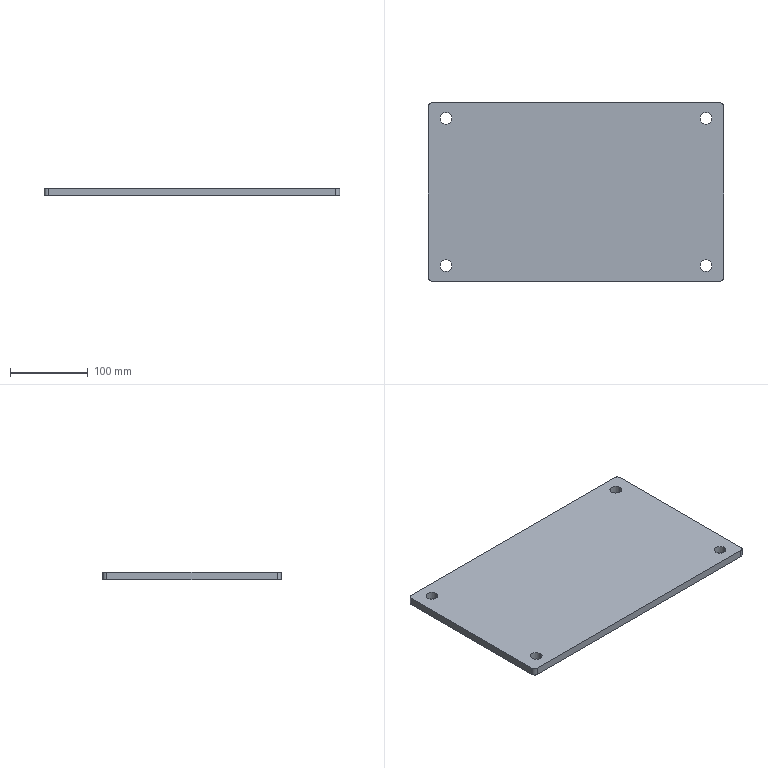Part | SolidWorks | features Chamfer 1, Extrusion 1, Fillet 1, HoleWzd 1 | 1 solid | 18 faces | box 381 x 230 x 10 mm | volume 869017 mm3 | cylinder 12 | plane 6 | commonest cylinder face diameters 15 x8 10 x4
STEP:
#1=CARTESIAN_POINT('',(-175.,95.,-5.));
#2=VERTEX_POINT('',#1);
#3=CARTESIAN_POINT('',(-160.,95.,-5.));
#4=VERTEX_POINT('',#3);
#5=CARTESIAN_POINT('',(-167.5,95.,-5.));
#6=DIRECTION('',(0.,0.,1.));
#7=DIRECTION('',(1.,0.,0.));
#8=AXIS2_PLACEMENT_3D('',#5,#6,#7);
#9=CIRCLE('',#8,7.5);
#10=EDGE_CURVE('',#2,#4,#9,.T.);
#11=ORIENTED_EDGE('',*,*,#10,.F.);
#12=CARTESIAN_POINT('',(-175.,95.,5.));
#13=VERTEX_POINT('',#12);
#14=CARTESIAN_POINT('',(-175.,95.,5.));
#15=DIRECTION('',(0.,0.,1.));
#16=VECTOR('',#15,1000.);
#17=LINE('',#14,#16);
#18=EDGE_CURVE('',#2,#13,#17,.T.);
#19=ORIENTED_EDGE('',*,*,#18,.T.);
#20=CARTESIAN_POINT('',(-160.,95.,5.));
#21=VERTEX_POINT('',#20);
#22=CARTESIAN_POINT('',(-167.5,95.,5.));
#23=DIRECTION('',(0.,0.,1.));
#24=DIRECTION('',(1.,0.,0.));
#25=AXIS2_PLACEMENT_3D('',#22,#23,#24);
#26=CIRCLE('',#25,7.5);
#27=EDGE_CURVE('',#13,#21,#26,.T.);
#28=ORIENTED_EDGE('',*,*,#27,.T.);
#29=CARTESIAN_POINT('',(-160.,95.,5.));
#30=DIRECTION('',(0.,0.,1.));
#31=VECTOR('',#30,1000.);
#32=LINE('',#29,#31);
#33=EDGE_CURVE('',#4,#21,#32,.T.);
#34=ORIENTED_EDGE('',*,*,#33,.F.);
#35=EDGE_LOOP('',(#11,#19,#28,#34));
#36=FACE_OUTER_BOUND('',#35,.T.);
#37=CARTESIAN_POINT('',(-167.5,95.,5.));
#38=DIRECTION('',(0.,0.,1.));
#39=DIRECTION('',(1.,0.,0.));
#40=AXIS2_PLACEMENT_3D('',#37,#38,#39);
#41=CYLINDRICAL_SURFACE('',#40,7.5);
#42=ADVANCED_FACE('',(#36),#41,.F.);
#43=CARTESIAN_POINT('',(160.,95.,-5.));
#44=VERTEX_POINT('',#43);
#45=CARTESIAN_POINT('',(175.,95.,-5.));
#46=VERTEX_POINT('',#45);
#47=CARTESIAN_POINT('',(167.5,95.,-5.));
#48=DIRECTION('',(0.,0.,1.));
#49=DIRECTION('',(1.,0.,0.));
#50=AXIS2_PLACEMENT_3D('',#47,#48,#49);
#51=CIRCLE('',#50,7.5);
#52=EDGE_CURVE('',#44,#46,#51,.T.);
#53=ORIENTED_EDGE('',*,*,#52,.F.);
#54=CARTESIAN_POINT('',(160.,95.,5.));
#55=VERTEX_POINT('',#54);
#56=CARTESIAN_POINT('',(160.,95.,5.));
#57=DIRECTION('',(0.,0.,1.));
#58=VECTOR('',#57,1000.);
#59=LINE('',#56,#58);
#60=EDGE_CURVE('',#44,#55,#59,.T.);
#61=ORIENTED_EDGE('',*,*,#60,.T.);
#62=CARTESIAN_POINT('',(175.,95.,5.));
#63=VERTEX_POINT('',#62);
#64=CARTESIAN_POINT('',(167.5,95.,5.));
#65=DIRECTION('',(0.,0.,1.));
#66=DIRECTION('',(1.,0.,0.));
#67=AXIS2_PLACEMENT_3D('',#64,#65,#66);
#68=CIRCLE('',#67,7.5);
#69=EDGE_CURVE('',#55,#63,#68,.T.);
#70=ORIENTED_EDGE('',*,*,#69,.T.);
#71=CARTESIAN_POINT('',(175.,95.,5.));
#72=DIRECTION('',(0.,0.,1.));
#73=VECTOR('',#72,1000.);
#74=LINE('',#71,#73);
#75=EDGE_CURVE('',#46,#63,#74,.T.);
#76=ORIENTED_EDGE('',*,*,#75,.F.);
#77=EDGE_LOOP('',(#53,#61,#70,#76));
#78=FACE_OUTER_BOUND('',#77,.T.);
#79=CARTESIAN_POINT('',(167.5,95.,5.));
#80=DIRECTION('',(0.,0.,1.));
#81=DIRECTION('',(1.,0.,0.));
#82=AXIS2_PLACEMENT_3D('',#79,#80,#81);
#83=CYLINDRICAL_SURFACE('',#82,7.5);
#84=ADVANCED_FACE('',(#78),#83,.F.);
#85=CARTESIAN_POINT('',(160.,-95.,-5.));
#86=VERTEX_POINT('',#85);
#87=CARTESIAN_POINT('',(175.,-95.,-5.));
#88=VERTEX_POINT('',#87);
#89=CARTESIAN_POINT('',(167.5,-95.,-5.));
#90=DIRECTION('',(0.,0.,1.));
#91=DIRECTION('',(1.,0.,0.));
#92=AXIS2_PLACEMENT_3D('',#89,#90,#91);
#93=CIRCLE('',#92,7.5);
#94=EDGE_CURVE('',#86,#88,#93,.T.);
#95=ORIENTED_EDGE('',*,*,#94,.F.);
#96=CARTESIAN_POINT('',(160.,-95.,5.));
#97=VERTEX_POINT('',#96);
#98=CARTESIAN_POINT('',(160.,-95.,5.));
#99=DIRECTION('',(0.,0.,1.));
#100=VECTOR('',#99,1000.);
#101=LINE('',#98,#100);
#102=EDGE_CURVE('',#86,#97,#101,.T.);
#103=ORIENTED_EDGE('',*,*,#102,.T.);
#104=CARTESIAN_POINT('',(175.,-95.,5.));
#105=VERTEX_POINT('',#104);
#106=CARTESIAN_POINT('',(167.5,-95.,5.));
#107=DIRECTION('',(0.,0.,1.));
#108=DIRECTION('',(1.,0.,0.));
#109=AXIS2_PLACEMENT_3D('',#106,#107,#108);
#110=CIRCLE('',#109,7.5);
#111=EDGE_CURVE('',#97,#105,#110,.T.);
#112=ORIENTED_EDGE('',*,*,#111,.T.);
#113=CARTESIAN_POINT('',(175.,-95.,5.));
#114=DIRECTION('',(0.,0.,1.));
#115=VECTOR('',#114,1000.);
#116=LINE('',#113,#115);
#117=EDGE_CURVE('',#88,#105,#116,.T.);
#118=ORIENTED_EDGE('',*,*,#117,.F.);
#119=EDGE_LOOP('',(#95,#103,#112,#118));
#120=FACE_OUTER_BOUND('',#119,.T.);
#121=CARTESIAN_POINT('',(167.5,-95.,5.));
#122=DIRECTION('',(0.,0.,1.));
#123=DIRECTION('',(1.,0.,0.));
#124=AXIS2_PLACEMENT_3D('',#121,#122,#123);
#125=CYLINDRICAL_SURFACE('',#124,7.5);
#126=ADVANCED_FACE('',(#120),#125,.F.);
#127=CARTESIAN_POINT('',(-175.,-95.,-5.));
#128=VERTEX_POINT('',#127);
#129=CARTESIAN_POINT('',(-160.,-95.,-5.));
#130=VERTEX_POINT('',#129);
#131=CARTESIAN_POINT('',(-167.5,-95.,-5.));
#132=DIRECTION('',(0.,0.,1.));
#133=DIRECTION('',(1.,0.,0.));
#134=AXIS2_PLACEMENT_3D('',#131,#132,#133);
#135=CIRCLE('',#134,7.5);
#136=EDGE_CURVE('',#128,#130,#135,.T.);
#137=ORIENTED_EDGE('',*,*,#136,.F.);
#138=CARTESIAN_POINT('',(-175.,-95.,5.));
#139=VERTEX_POINT('',#138);
#140=CARTESIAN_POINT('',(-175.,-95.,5.));
#141=DIRECTION('',(0.,0.,1.));
#142=VECTOR('',#141,1000.);
#143=LINE('',#140,#142);
#144=EDGE_CURVE('',#128,#139,#143,.T.);
#145=ORIENTED_EDGE('',*,*,#144,.T.);
#146=CARTESIAN_POINT('',(-160.,-95.,5.));
#147=VERTEX_POINT('',#146);
#148=CARTESIAN_POINT('',(-167.5,-95.,5.));
#149=DIRECTION('',(0.,0.,1.));
#150=DIRECTION('',(1.,0.,0.));
#151=AXIS2_PLACEMENT_3D('',#148,#149,#150);
#152=CIRCLE('',#151,7.5);
#153=EDGE_CURVE('',#139,#147,#152,.T.);
#154=ORIENTED_EDGE('',*,*,#153,.T.);
#155=CARTESIAN_POINT('',(-160.,-95.,5.));
#156=DIRECTION('',(0.,0.,1.));
#157=VECTOR('',#156,1000.);
#158=LINE('',#155,#157);
#159=EDGE_CURVE('',#130,#147,#158,.T.);
#160=ORIENTED_EDGE('',*,*,#159,.F.);
#161=EDGE_LOOP('',(#137,#145,#154,#160));
#162=FACE_OUTER_BOUND('',#161,.T.);
#163=CARTESIAN_POINT('',(-167.5,-95.,5.));
#164=DIRECTION('',(0.,0.,1.));
#165=DIRECTION('',(1.,0.,0.));
#166=AXIS2_PLACEMENT_3D('',#163,#164,#165);
#167=CYLINDRICAL_SURFACE('',#166,7.5);
#168=ADVANCED_FACE('',(#162),#167,.F.);
#169=CARTESIAN_POINT('',(-190.5,110.,-5.));
#170=VERTEX_POINT('',#169);
#171=CARTESIAN_POINT('',(-190.5,-110.,-5.));
#172=VERTEX_POINT('',#171);
#173=CARTESIAN_POINT('',(-190.5,-115.,-5.));
#174=DIRECTION('',(0.,-1.,0.));
#175=VECTOR('',#174,1000.);
#176=LINE('',#173,#175);
#177=EDGE_CURVE('',#170,#172,#176,.T.);
#178=ORIENTED_EDGE('',*,*,#177,.T.);
#179=CARTESIAN_POINT('',(-190.5,-110.,5.));
#180=VERTEX_POINT('',#179);
#181=CARTESIAN_POINT('',(-190.5,-110.,5.));
#182=DIRECTION('',(0.,0.,1.));
#183=VECTOR('',#182,1000.);
#184=LINE('',#181,#183);
#185=EDGE_CURVE('',#172,#180,#184,.T.);
#186=ORIENTED_EDGE('',*,*,#185,.T.);
#187=CARTESIAN_POINT('',(-190.5,110.,5.));
#188=VERTEX_POINT('',#187);
#189=CARTESIAN_POINT('',(-190.5,-115.,5.));
#190=DIRECTION('',(0.,-1.,0.));
#191=VECTOR('',#190,1000.);
#192=LINE('',#189,#191);
#193=EDGE_CURVE('',#188,#180,#192,.T.);
#194=ORIENTED_EDGE('',*,*,#193,.F.);
#195=CARTESIAN_POINT('',(-190.5,110.,5.));
#196=DIRECTION('',(0.,0.,-1.));
#197=VECTOR('',#196,1000.);
#198=LINE('',#195,#197);
#199=EDGE_CURVE('',#188,#170,#198,.T.);
#200=ORIENTED_EDGE('',*,*,#199,.T.);
#201=EDGE_LOOP('',(#178,#186,#194,#200));
#202=FACE_OUTER_BOUND('',#201,.T.);
#203=CARTESIAN_POINT('',(-190.5,-115.,5.));
#204=DIRECTION('',(1.,0.,0.));
#205=DIRECTION('',(0.,0.,-1.));
#206=AXIS2_PLACEMENT_3D('',#203,#204,#205);
#207=PLANE('',#206);
#208=ADVANCED_FACE('',(#202),#207,.F.);
#209=CARTESIAN_POINT('',(-185.5,-115.,-5.));
#210=VERTEX_POINT('',#209);
#211=CARTESIAN_POINT('',(185.5,-115.,-5.));
#212=VERTEX_POINT('',#211);
#213=CARTESIAN_POINT('',(190.5,-115.,-5.));
#214=DIRECTION('',(1.,0.,0.));
#215=VECTOR('',#214,1000.);
#216=LINE('',#213,#215);
#217=EDGE_CURVE('',#210,#212,#216,.T.);
#218=ORIENTED_EDGE('',*,*,#217,.T.);
#219=CARTESIAN_POINT('',(185.5,-115.,5.));
#220=VERTEX_POINT('',#219);
#221=CARTESIAN_POINT('',(185.5,-115.,5.));
#222=DIRECTION('',(0.,0.,1.));
#223=VECTOR('',#222,1000.);
#224=LINE('',#221,#223);
#225=EDGE_CURVE('',#212,#220,#224,.T.);
#226=ORIENTED_EDGE('',*,*,#225,.T.);
#227=CARTESIAN_POINT('',(-185.5,-115.,5.));
#228=VERTEX_POINT('',#227);
#229=CARTESIAN_POINT('',(190.5,-115.,5.));
#230=DIRECTION('',(1.,0.,0.));
#231=VECTOR('',#230,1000.);
#232=LINE('',#229,#231);
#233=EDGE_CURVE('',#228,#220,#232,.T.);
#234=ORIENTED_EDGE('',*,*,#233,.F.);
#235=CARTESIAN_POINT('',(-185.5,-115.,5.));
#236=DIRECTION('',(0.,0.,-1.));
#237=VECTOR('',#236,1000.);
#238=LINE('',#235,#237);
#239=EDGE_CURVE('',#228,#210,#238,.T.);
#240=ORIENTED_EDGE('',*,*,#239,.T.);
#241=EDGE_LOOP('',(#218,#226,#234,#240));
#242=FACE_OUTER_BOUND('',#241,.T.);
#243=CARTESIAN_POINT('',(190.5,-115.,5.));
#244=DIRECTION('',(0.,1.,0.));
#245=DIRECTION('',(-1.,0.,0.));
#246=AXIS2_PLACEMENT_3D('',#243,#244,#245);
#247=PLANE('',#246);
#248=ADVANCED_FACE('',(#242),#247,.F.);
#249=CARTESIAN_POINT('',(190.5,-110.,-5.));
#250=VERTEX_POINT('',#249);
#251=CARTESIAN_POINT('',(190.5,110.,-5.));
#252=VERTEX_POINT('',#251);
#253=CARTESIAN_POINT('',(190.5,-115.,-5.));
#254=DIRECTION('',(0.,1.,0.));
#255=VECTOR('',#254,1000.);
#256=LINE('',#253,#255);
#257=EDGE_CURVE('',#250,#252,#256,.T.);
#258=ORIENTED_EDGE('',*,*,#257,.T.);
#259=CARTESIAN_POINT('',(190.5,110.,5.));
#260=VERTEX_POINT('',#259);
#261=CARTESIAN_POINT('',(190.5,110.,5.));
#262=DIRECTION('',(0.,0.,1.));
#263=VECTOR('',#262,1000.);
#264=LINE('',#261,#263);
#265=EDGE_CURVE('',#252,#260,#264,.T.);
#266=ORIENTED_EDGE('',*,*,#265,.T.);
#267=CARTESIAN_POINT('',(190.5,-110.,5.));
#268=VERTEX_POINT('',#267);
#269=CARTESIAN_POINT('',(190.5,-115.,5.));
#270=DIRECTION('',(0.,1.,0.));
#271=VECTOR('',#270,1000.);
#272=LINE('',#269,#271);
#273=EDGE_CURVE('',#268,#260,#272,.T.);
#274=ORIENTED_EDGE('',*,*,#273,.F.);
#275=CARTESIAN_POINT('',(190.5,-110.,5.));
#276=DIRECTION('',(0.,0.,-1.));
#277=VECTOR('',#276,1000.);
#278=LINE('',#275,#277);
#279=EDGE_CURVE('',#268,#250,#278,.T.);
#280=ORIENTED_EDGE('',*,*,#279,.T.);
#281=EDGE_LOOP('',(#258,#266,#274,#280));
#282=FACE_OUTER_BOUND('',#281,.T.);
#283=CARTESIAN_POINT('',(190.5,-115.,5.));
#284=DIRECTION('',(-1.,0.,0.));
#285=DIRECTION('',(0.,0.,1.));
#286=AXIS2_PLACEMENT_3D('',#283,#284,#285);
#287=PLANE('',#286);
#288=ADVANCED_FACE('',(#282),#287,.F.);
#289=CARTESIAN_POINT('',(185.5,115.,5.));
#290=VERTEX_POINT('',#289);
#291=CARTESIAN_POINT('',(-185.5,115.,5.));
#292=VERTEX_POINT('',#291);
#293=CARTESIAN_POINT('',(190.5,115.,5.));
#294=DIRECTION('',(-1.,0.,0.));
#295=VECTOR('',#294,1000.);
#296=LINE('',#293,#295);
#297=EDGE_CURVE('',#290,#292,#296,.T.);
#298=ORIENTED_EDGE('',*,*,#297,.F.);
#299=CARTESIAN_POINT('',(185.5,115.,-5.));
#300=VERTEX_POINT('',#299);
#301=CARTESIAN_POINT('',(185.5,115.,5.));
#302=DIRECTION('',(0.,0.,-1.));
#303=VECTOR('',#302,1000.);
#304=LINE('',#301,#303);
#305=EDGE_CURVE('',#290,#300,#304,.T.);
#306=ORIENTED_EDGE('',*,*,#305,.T.);
#307=CARTESIAN_POINT('',(-185.5,115.,-5.));
#308=VERTEX_POINT('',#307);
#309=CARTESIAN_POINT('',(190.5,115.,-5.));
#310=DIRECTION('',(-1.,0.,0.));
#311=VECTOR('',#310,1000.);
#312=LINE('',#309,#311);
#313=EDGE_CURVE('',#300,#308,#312,.T.);
#314=ORIENTED_EDGE('',*,*,#313,.T.);
#315=CARTESIAN_POINT('',(-185.5,115.,5.));
#316=DIRECTION('',(0.,0.,1.));
#317=VECTOR('',#316,1000.);
#318=LINE('',#315,#317);
#319=EDGE_CURVE('',#308,#292,#318,.T.);
#320=ORIENTED_EDGE('',*,*,#319,.T.);
#321=EDGE_LOOP('',(#298,#306,#314,#320));
#322=FACE_OUTER_BOUND('',#321,.T.);
#323=CARTESIAN_POINT('',(190.5,115.,5.));
#324=DIRECTION('',(0.,-1.,0.));
#325=DIRECTION('',(1.,0.,0.));
#326=AXIS2_PLACEMENT_3D('',#323,#324,#325);
#327=PLANE('',#326);
#328=ADVANCED_FACE('',(#322),#327,.F.);
#329=CARTESIAN_POINT('',(-167.5,95.,5.));
#330=DIRECTION('',(0.,0.,1.));
#331=DIRECTION('',(1.,0.,0.));
#332=AXIS2_PLACEMENT_3D('',#329,#330,#331);
#333=CIRCLE('',#332,7.5);
#334=EDGE_CURVE('',#21,#13,#333,.T.);
#335=ORIENTED_EDGE('',*,*,#334,.F.);
#336=ORIENTED_EDGE('',*,*,#27,.F.);
#337=EDGE_LOOP('',(#335,#336));
#338=FACE_BOUND('',#337,.T.);
#339=CARTESIAN_POINT('',(167.5,95.,5.));
#340=DIRECTION('',(0.,0.,1.));
#341=DIRECTION('',(1.,0.,0.));
#342=AXIS2_PLACEMENT_3D('',#339,#340,#341);
#343=CIRCLE('',#342,7.5);
#344=EDGE_CURVE('',#63,#55,#343,.T.);
#345=ORIENTED_EDGE('',*,*,#344,.F.);
#346=ORIENTED_EDGE('',*,*,#69,.F.);
#347=EDGE_LOOP('',(#345,#346));
#348=FACE_BOUND('',#347,.T.);
#349=CARTESIAN_POINT('',(167.5,-95.,5.));
#350=DIRECTION('',(0.,0.,1.));
#351=DIRECTION('',(1.,0.,0.));
#352=AXIS2_PLACEMENT_3D('',#349,#350,#351);
#353=CIRCLE('',#352,7.5);
#354=EDGE_CURVE('',#105,#97,#353,.T.);
#355=ORIENTED_EDGE('',*,*,#354,.F.);
#356=ORIENTED_EDGE('',*,*,#111,.F.);
#357=EDGE_LOOP('',(#355,#356));
#358=FACE_BOUND('',#357,.T.);
#359=CARTESIAN_POINT('',(-167.5,-95.,5.));
#360=DIRECTION('',(0.,0.,1.));
#361=DIRECTION('',(1.,0.,0.));
#362=AXIS2_PLACEMENT_3D('',#359,#360,#361);
#363=CIRCLE('',#362,7.5);
#364=EDGE_CURVE('',#147,#139,#363,.T.);
#365=ORIENTED_EDGE('',*,*,#364,.F.);
#366=ORIENTED_EDGE('',*,*,#153,.F.);
#367=EDGE_LOOP('',(#365,#366));
#368=FACE_BOUND('',#367,.T.);
#369=ORIENTED_EDGE('',*,*,#273,.T.);
#370=CARTESIAN_POINT('',(185.5,110.,5.));
#371=DIRECTION('',(0.,0.,1.));
#372=DIRECTION('',(1.,0.,0.));
#373=AXIS2_PLACEMENT_3D('',#370,#371,#372);
#374=CIRCLE('',#373,5.);
#375=EDGE_CURVE('',#260,#290,#374,.T.);
#376=ORIENTED_EDGE('',*,*,#375,.T.);
#377=ORIENTED_EDGE('',*,*,#297,.T.);
#378=CARTESIAN_POINT('',(-185.5,110.,5.));
#379=DIRECTION('',(0.,0.,1.));
#380=DIRECTION('',(1.,0.,0.));
#381=AXIS2_PLACEMENT_3D('',#378,#379,#380);
#382=CIRCLE('',#381,5.);
#383=EDGE_CURVE('',#292,#188,#382,.T.);
#384=ORIENTED_EDGE('',*,*,#383,.T.);
#385=ORIENTED_EDGE('',*,*,#193,.T.);
#386=CARTESIAN_POINT('',(-185.5,-110.,5.));
#387=DIRECTION('',(0.,0.,1.));
#388=DIRECTION('',(1.,0.,0.));
#389=AXIS2_PLACEMENT_3D('',#386,#387,#388);
#390=CIRCLE('',#389,5.);
#391=EDGE_CURVE('',#180,#228,#390,.T.);
#392=ORIENTED_EDGE('',*,*,#391,.T.);
#393=ORIENTED_EDGE('',*,*,#233,.T.);
#394=CARTESIAN_POINT('',(185.5,-110.,5.));
#395=DIRECTION('',(0.,0.,1.));
#396=DIRECTION('',(1.,0.,0.));
#397=AXIS2_PLACEMENT_3D('',#394,#395,#396);
#398=CIRCLE('',#397,5.);
#399=EDGE_CURVE('',#220,#268,#398,.T.);
#400=ORIENTED_EDGE('',*,*,#399,.T.);
#401=EDGE_LOOP('',(#369,#376,#377,#384,#385,#392,#393,#400));
#402=FACE_OUTER_BOUND('',#401,.T.);
#403=CARTESIAN_POINT('',(0.,0.,5.));
#404=DIRECTION('',(0.,0.,1.));
#405=DIRECTION('',(1.,0.,0.));
#406=AXIS2_PLACEMENT_3D('',#403,#404,#405);
#407=PLANE('',#406);
#408=ADVANCED_FACE('',(#338,#348,#358,#368,#402),#407,.T.);
#409=CARTESIAN_POINT('',(-167.5,95.,-5.));
#410=DIRECTION('',(0.,0.,1.));
#411=DIRECTION('',(1.,0.,0.));
#412=AXIS2_PLACEMENT_3D('',#409,#410,#411);
#413=CIRCLE('',#412,7.5);
#414=EDGE_CURVE('',#4,#2,#413,.T.);
#415=ORIENTED_EDGE('',*,*,#414,.T.);
#416=ORIENTED_EDGE('',*,*,#10,.T.);
#417=EDGE_LOOP('',(#415,#416));
#418=FACE_BOUND('',#417,.T.);
#419=CARTESIAN_POINT('',(167.5,95.,-5.));
#420=DIRECTION('',(0.,0.,1.));
#421=DIRECTION('',(1.,0.,0.));
#422=AXIS2_PLACEMENT_3D('',#419,#420,#421);
#423=CIRCLE('',#422,7.5);
#424=EDGE_CURVE('',#46,#44,#423,.T.);
#425=ORIENTED_EDGE('',*,*,#424,.T.);
#426=ORIENTED_EDGE('',*,*,#52,.T.);
#427=EDGE_LOOP('',(#425,#426));
#428=FACE_BOUND('',#427,.T.);
#429=CARTESIAN_POINT('',(167.5,-95.,-5.));
#430=DIRECTION('',(0.,0.,1.));
#431=DIRECTION('',(1.,0.,0.));
#432=AXIS2_PLACEMENT_3D('',#429,#430,#431);
#433=CIRCLE('',#432,7.5);
#434=EDGE_CURVE('',#88,#86,#433,.T.);
#435=ORIENTED_EDGE('',*,*,#434,.T.);
#436=ORIENTED_EDGE('',*,*,#94,.T.);
#437=EDGE_LOOP('',(#435,#436));
#438=FACE_BOUND('',#437,.T.);
#439=CARTESIAN_POINT('',(-167.5,-95.,-5.));
#440=DIRECTION('',(0.,0.,1.));
#441=DIRECTION('',(1.,0.,0.));
#442=AXIS2_PLACEMENT_3D('',#439,#440,#441);
#443=CIRCLE('',#442,7.5);
#444=EDGE_CURVE('',#130,#128,#443,.T.);
#445=ORIENTED_EDGE('',*,*,#444,.T.);
#446=ORIENTED_EDGE('',*,*,#136,.T.);
#447=EDGE_LOOP('',(#445,#446));
#448=FACE_BOUND('',#447,.T.);
#449=ORIENTED_EDGE('',*,*,#313,.F.);
#450=CARTESIAN_POINT('',(185.5,110.,-5.));
#451=DIRECTION('',(0.,0.,-1.));
#452=DIRECTION('',(1.,0.,0.));
#453=AXIS2_PLACEMENT_3D('',#450,#451,#452);
#454=CIRCLE('',#453,5.);
#455=EDGE_CURVE('',#300,#252,#454,.T.);
#456=ORIENTED_EDGE('',*,*,#455,.T.);
#457=ORIENTED_EDGE('',*,*,#257,.F.);
#458=CARTESIAN_POINT('',(185.5,-110.,-5.));
#459=DIRECTION('',(0.,0.,-1.));
#460=DIRECTION('',(1.,0.,0.));
#461=AXIS2_PLACEMENT_3D('',#458,#459,#460);
#462=CIRCLE('',#461,5.);
#463=EDGE_CURVE('',#250,#212,#462,.T.);
#464=ORIENTED_EDGE('',*,*,#463,.T.);
#465=ORIENTED_EDGE('',*,*,#217,.F.);
#466=CARTESIAN_POINT('',(-185.5,-110.,-5.));
#467=DIRECTION('',(0.,0.,-1.));
#468=DIRECTION('',(1.,0.,0.));
#469=AXIS2_PLACEMENT_3D('',#466,#467,#468);
#470=CIRCLE('',#469,5.);
#471=EDGE_CURVE('',#210,#172,#470,.T.);
#472=ORIENTED_EDGE('',*,*,#471,.T.);
#473=ORIENTED_EDGE('',*,*,#177,.F.);
#474=CARTESIAN_POINT('',(-185.5,110.,-5.));
#475=DIRECTION('',(0.,0.,-1.));
#476=DIRECTION('',(1.,0.,0.));
#477=AXIS2_PLACEMENT_3D('',#474,#475,#476);
#478=CIRCLE('',#477,5.);
#479=EDGE_CURVE('',#170,#308,#478,.T.);
#480=ORIENTED_EDGE('',*,*,#479,.T.);
#481=EDGE_LOOP('',(#449,#456,#457,#464,#465,#472,#473,#480));
#482=FACE_OUTER_BOUND('',#481,.T.);
#483=CARTESIAN_POINT('',(0.,0.,-5.));
#484=DIRECTION('',(0.,0.,1.));
#485=DIRECTION('',(1.,0.,0.));
#486=AXIS2_PLACEMENT_3D('',#483,#484,#485);
#487=PLANE('',#486);
#488=ADVANCED_FACE('',(#418,#428,#438,#448,#482),#487,.F.);
#489=ORIENTED_EDGE('',*,*,#144,.F.);
#490=ORIENTED_EDGE('',*,*,#444,.F.);
#491=ORIENTED_EDGE('',*,*,#159,.T.);
#492=ORIENTED_EDGE('',*,*,#364,.T.);
#493=EDGE_LOOP('',(#489,#490,#491,#492));
#494=FACE_OUTER_BOUND('',#493,.T.);
#495=CARTESIAN_POINT('',(-167.5,-95.,5.));
#496=DIRECTION('',(0.,0.,1.));
#497=DIRECTION('',(1.,0.,0.));
#498=AXIS2_PLACEMENT_3D('',#495,#496,#497);
#499=CYLINDRICAL_SURFACE('',#498,7.5);
#500=ADVANCED_FACE('',(#494),#499,.F.);
#501=ORIENTED_EDGE('',*,*,#102,.F.);
#502=ORIENTED_EDGE('',*,*,#434,.F.);
#503=ORIENTED_EDGE('',*,*,#117,.T.);
#504=ORIENTED_EDGE('',*,*,#354,.T.);
#505=EDGE_LOOP('',(#501,#502,#503,#504));
#506=FACE_OUTER_BOUND('',#505,.T.);
#507=CARTESIAN_POINT('',(167.5,-95.,5.));
#508=DIRECTION('',(0.,0.,1.));
#509=DIRECTION('',(1.,0.,0.));
#510=AXIS2_PLACEMENT_3D('',#507,#508,#509);
#511=CYLINDRICAL_SURFACE('',#510,7.5);
#512=ADVANCED_FACE('',(#506),#511,.F.);
#513=ORIENTED_EDGE('',*,*,#60,.F.);
#514=ORIENTED_EDGE('',*,*,#424,.F.);
#515=ORIENTED_EDGE('',*,*,#75,.T.);
#516=ORIENTED_EDGE('',*,*,#344,.T.);
#517=EDGE_LOOP('',(#513,#514,#515,#516));
#518=FACE_OUTER_BOUND('',#517,.T.);
#519=CARTESIAN_POINT('',(167.5,95.,5.));
#520=DIRECTION('',(0.,0.,1.));
#521=DIRECTION('',(1.,0.,0.));
#522=AXIS2_PLACEMENT_3D('',#519,#520,#521);
#523=CYLINDRICAL_SURFACE('',#522,7.5);
#524=ADVANCED_FACE('',(#518),#523,.F.);
#525=ORIENTED_EDGE('',*,*,#18,.F.);
#526=ORIENTED_EDGE('',*,*,#414,.F.);
#527=ORIENTED_EDGE('',*,*,#33,.T.);
#528=ORIENTED_EDGE('',*,*,#334,.T.);
#529=EDGE_LOOP('',(#525,#526,#527,#528));
#530=FACE_OUTER_BOUND('',#529,.T.);
#531=CARTESIAN_POINT('',(-167.5,95.,5.));
#532=DIRECTION('',(0.,0.,1.));
#533=DIRECTION('',(1.,0.,0.));
#534=AXIS2_PLACEMENT_3D('',#531,#532,#533);
#535=CYLINDRICAL_SURFACE('',#534,7.5);
#536=ADVANCED_FACE('',(#530),#535,.F.);
#537=ORIENTED_EDGE('',*,*,#375,.F.);
#538=ORIENTED_EDGE('',*,*,#265,.F.);
#539=ORIENTED_EDGE('',*,*,#455,.F.);
#540=ORIENTED_EDGE('',*,*,#305,.F.);
#541=EDGE_LOOP('',(#537,#538,#539,#540));
#542=FACE_OUTER_BOUND('',#541,.T.);
#543=CARTESIAN_POINT('',(185.5,110.,5.));
#544=DIRECTION('',(0.,0.,-1.));
#545=DIRECTION('',(-1.,0.,0.));
#546=AXIS2_PLACEMENT_3D('',#543,#544,#545);
#547=CYLINDRICAL_SURFACE('',#546,5.);
#548=ADVANCED_FACE('',(#542),#547,.T.);
#549=ORIENTED_EDGE('',*,*,#399,.F.);
#550=ORIENTED_EDGE('',*,*,#225,.F.);
#551=ORIENTED_EDGE('',*,*,#463,.F.);
#552=ORIENTED_EDGE('',*,*,#279,.F.);
#553=EDGE_LOOP('',(#549,#550,#551,#552));
#554=FACE_OUTER_BOUND('',#553,.T.);
#555=CARTESIAN_POINT('',(185.5,-110.,5.));
#556=DIRECTION('',(0.,0.,-1.));
#557=DIRECTION('',(-1.,0.,0.));
#558=AXIS2_PLACEMENT_3D('',#555,#556,#557);
#559=CYLINDRICAL_SURFACE('',#558,5.);
#560=ADVANCED_FACE('',(#554),#559,.T.);
#561=ORIENTED_EDGE('',*,*,#391,.F.);
#562=ORIENTED_EDGE('',*,*,#185,.F.);
#563=ORIENTED_EDGE('',*,*,#471,.F.);
#564=ORIENTED_EDGE('',*,*,#239,.F.);
#565=EDGE_LOOP('',(#561,#562,#563,#564));
#566=FACE_OUTER_BOUND('',#565,.T.);
#567=CARTESIAN_POINT('',(-185.5,-110.,5.));
#568=DIRECTION('',(0.,0.,-1.));
#569=DIRECTION('',(-1.,0.,0.));
#570=AXIS2_PLACEMENT_3D('',#567,#568,#569);
#571=CYLINDRICAL_SURFACE('',#570,5.);
#572=ADVANCED_FACE('',(#566),#571,.T.);
#573=ORIENTED_EDGE('',*,*,#383,.F.);
#574=ORIENTED_EDGE('',*,*,#319,.F.);
#575=ORIENTED_EDGE('',*,*,#479,.F.);
#576=ORIENTED_EDGE('',*,*,#199,.F.);
#577=EDGE_LOOP('',(#573,#574,#575,#576));
#578=FACE_OUTER_BOUND('',#577,.T.);
#579=CARTESIAN_POINT('',(-185.5,110.,5.));
#580=DIRECTION('',(0.,0.,-1.));
#581=DIRECTION('',(-1.,0.,0.));
#582=AXIS2_PLACEMENT_3D('',#579,#580,#581);
#583=CYLINDRICAL_SURFACE('',#582,5.);
#584=ADVANCED_FACE('',(#578),#583,.T.);
#585=CLOSED_SHELL('',(#42,#84,#126,#168,#208,#248,#288,#328,#408,#488,#500,#512,#524,#536,#548,#560,#572,#584));
#586=MANIFOLD_SOLID_BREP('',#585);
#587=CARTESIAN_POINT('',(0.,0.,0.));
#588=DIRECTION('',(0.,0.,1.));
#589=DIRECTION('',(1.,0.,0.));
#590=AXIS2_PLACEMENT_3D('',#587,#588,#589);
#591=(LENGTH_UNIT()NAMED_UNIT(*)SI_UNIT(.MILLI.,.METRE.));
#592=UNCERTAINTY_MEASURE_WITH_UNIT(LENGTH_MEASURE(0.00001),#591,'','');
#593=(NAMED_UNIT(*)PLANE_ANGLE_UNIT()SI_UNIT($,.RADIAN.));
#594=(NAMED_UNIT(*)SI_UNIT($,.STERADIAN.)SOLID_ANGLE_UNIT());
#595=(GEOMETRIC_REPRESENTATION_CONTEXT(3)GLOBAL_UNCERTAINTY_ASSIGNED_CONTEXT((#592))GLOBAL_UNIT_ASSIGNED_CONTEXT((#591,#593,#594))REPRESENTATION_CONTEXT('',''));
#596=ADVANCED_BREP_SHAPE_REPRESENTATION('',(#586,#590),#595);